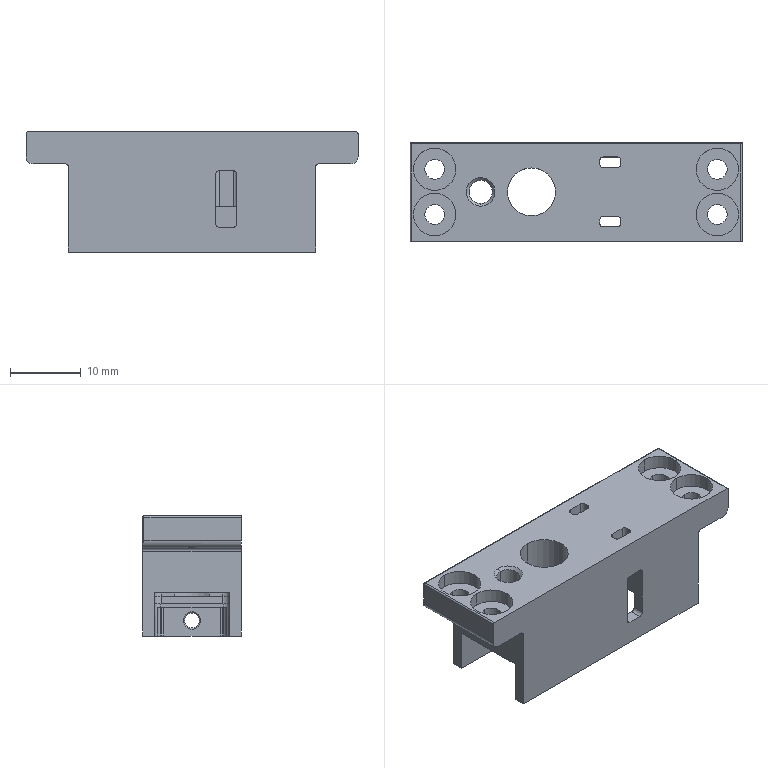NC program | NX | posted with a generic post | part box 47 x 14 x 17 mm
Lines 365 to 2938 of 2938, first 2161 of 2566 lines:
(ZLEVEL_PROFILE_COPY_1_COPY , TOOL : D1)
N686 T22 M6
N688 G54
N690 G17 G0 G90 X5.076 Y4.45 B0. C0. S9500 M3
N692 G43 Z30. H22
N694 Z1.
N696 G94 G1 X3.85 Z0.936 F1000.
N698 Y3.95 Z0.91
N700 X5.85 Z0.805
N702 Y4.45 Z0.779
N704 X3.85 Z0.674
N706 Y3.95 Z0.648
N708 X5.85 Z0.543
N710 Y4.45 Z0.516
N712 X3.85 Z0.412
N714 Y3.95 Z0.385
N716 X5.85 Z0.281
N718 Y4.45 Z0.254
N720 X3.85 Z0.15
N722 Y3.95 Z0.123
N724 X5.85 Z0.019
N726 Y4.45 Z-0.008
N728 X4.85 Z-0.06
N730 X3.85 F850.
N732 Y3.95
N734 X5.85
N736 Y4.45
N738 X4.85
N740 X3.85 Z-0.077
N742 Y4.075 Z-0.084
N744 X3.849 Y3.949 Z-0.086
N746 X3.931 Y3.95 Z-0.088
N748 X5.787 Z-0.12
N750 X5.85
N752 Y4.45
N754 X4.85
N756 X3.85 Z-0.137
N758 Y4.075 Z-0.144
N760 X3.849 Y3.949 Z-0.146
N762 X3.931 Y3.95 Z-0.148
N764 X5.787 Z-0.18
N766 X5.85
N768 Y4.45
N770 X4.85
N772 X3.85 Z-0.197
N774 Y4.075 Z-0.204
N776 X3.849 Y3.949 Z-0.206
N778 X3.931 Y3.95 Z-0.208
N780 X5.787 Z-0.24
N782 X5.85
N784 Y4.45
N786 X4.85
N788 X3.85 Z-0.257
N790 Y4.075 Z-0.264
N792 X3.849 Y3.949 Z-0.266
N794 X3.931 Y3.95 Z-0.268
N796 X5.787 Z-0.3
N798 X5.85
N800 Y4.45
N802 X4.85
N804 X3.85 Z-0.317
N806 Y4.075 Z-0.324
N808 X3.849 Y3.949 Z-0.326
N810 X3.931 Y3.95 Z-0.328
N812 X5.787 Z-0.36
N814 X5.85
N816 Y4.45
N818 X4.85
N820 X3.85 Z-0.377
N822 Y4.075 Z-0.384
N824 X3.849 Y3.949 Z-0.386
N826 X3.931 Y3.95 Z-0.388
N828 X5.787 Z-0.42
N830 X5.85
N832 Y4.45
N834 X4.85
N836 X3.85 Z-0.437
N838 Y4.075 Z-0.444
N840 X3.849 Y3.949 Z-0.446
N842 X3.931 Y3.95 Z-0.448
N844 X5.787 Z-0.48
N846 X5.85
N848 Y4.45
N850 X4.85
N852 X3.85 Z-0.497
N854 Y4.075 Z-0.504
N856 X3.849 Y3.949 Z-0.506
N858 X3.931 Y3.95 Z-0.508
N860 X5.787 Z-0.54
N862 X5.85
N864 Y4.45
N866 X4.85
N868 X3.85 Z-0.557
N870 Y4.075 Z-0.564
N872 X3.849 Y3.949 Z-0.566
N874 X3.931 Y3.95 Z-0.568
N876 X5.787 Z-0.6
N878 X5.85
N880 Y4.45
N882 X4.85
N884 X3.85 Z-0.617
N886 Y4.075 Z-0.624
N888 X3.849 Y3.949 Z-0.626
N890 X3.931 Y3.95 Z-0.628
N892 X5.787 Z-0.66
N894 X5.85
N896 Y4.45
N898 X4.85
N900 X3.85 Z-0.677
N902 Y4.075 Z-0.684
N904 X3.849 Y3.949 Z-0.686
N906 X3.931 Y3.95 Z-0.688
N908 X5.787 Z-0.72
N910 X5.85
N912 Y4.45
N914 X4.85
N916 X3.85 Z-0.737
N918 Y4.075 Z-0.744
N920 X3.849 Y3.949 Z-0.746
N922 X3.931 Y3.95 Z-0.748
N924 X5.787 Z-0.78
N926 X5.85
N928 Y4.45
N930 X4.85
N932 X3.85 Z-0.797
N934 Y4.075 Z-0.804
N936 X3.849 Y3.949 Z-0.806
N938 X3.931 Y3.95 Z-0.808
N940 X5.787 Z-0.84
N942 X5.85
N944 Y4.45
N946 X4.85
N948 X3.85 Z-0.857
N950 Y4.075 Z-0.864
N952 X3.849 Y3.949 Z-0.866
N954 X3.931 Y3.95 Z-0.868
N956 X5.787 Z-0.9
N958 X5.85
N960 Y4.45
N962 X4.85
N964 X3.85 Z-0.917
N966 Y4.075 Z-0.924
N968 X3.849 Y3.949 Z-0.926
N970 X3.931 Y3.95 Z-0.928
N972 X5.787 Z-0.96
N974 X5.85
N976 Y4.45
N978 X4.85
N980 X3.85 Z-0.977
N982 Y4.075 Z-0.984
N984 Y3.95 Z-0.986
N986 X3.931 Z-0.988
N988 X5.787 Z-1.02
N990 X5.85
N992 Y4.45
N994 X4.85
N996 X3.85 Z-1.037
N998 Y4.075 Z-1.044
N1000 Y3.95 Z-1.046
N1002 X3.931 Z-1.048
N1004 X5.787 Z-1.08
N1006 X5.85
N1008 Y4.45
N1010 X4.85
N1012 X3.85 Z-1.097
N1014 Y4.075 Z-1.104
N1016 Y3.95 Z-1.106
N1018 X3.931 Z-1.108
N1020 X5.787 Z-1.14
N1022 X5.85
N1024 Y4.45
N1026 X4.85
N1028 X3.85 Z-1.157
N1030 Y4.075 Z-1.164
N1032 Y3.95 Z-1.166
N1034 X3.931 Z-1.168
N1036 X5.787 Z-1.2
N1038 X5.85
N1040 Y4.45
N1042 X4.85
N1044 X3.85 Z-1.217
N1046 Y4.075 Z-1.224
N1048 Y3.95 Z-1.226
N1050 X3.931 Z-1.228
N1052 X5.787 Z-1.26
N1054 X5.84
N1056 X5.85 Y3.978
N1058 Y4.45
N1060 X4.85
N1062 X3.85 Z-1.277
N1064 Y4.075 Z-1.284
N1066 Y3.95 Z-1.286
N1068 X3.931 Z-1.288
N1070 X5.787 Z-1.32
N1072 X5.84
N1074 X5.85 Y3.978
N1076 Y4.45
N1078 X4.85
N1080 X3.85 Z-1.337
N1082 Y4.075 Z-1.344
N1084 Y3.95 Z-1.346
N1086 X3.931 Z-1.348
N1088 X5.787 Z-1.38
N1090 X5.84
N1092 X5.85 Y3.978
N1094 Y4.45
N1096 X4.85
N1098 X3.85 Z-1.397
N1100 Y4.075 Z-1.404
N1102 Y3.95 Z-1.406
N1104 X3.931 Z-1.408
N1106 X5.787 Z-1.44
N1108 X5.84
N1110 X5.85 Y3.978
N1112 Y4.45
N1114 X4.85
N1116 X3.85 Z-1.457
N1118 Y4.075 Z-1.464
N1120 Y3.95 Z-1.466
N1122 X3.931 Z-1.468
N1124 X5.787 Z-1.5
N1126 X5.84
N1128 X5.85 Y3.978
N1130 Y4.45
N1132 X4.85
N1134 X3.85 Z-1.517
N1136 Y4.075 Z-1.524
N1138 Y3.95 Z-1.526
N1140 X3.931 Z-1.528
N1142 X5.787 Z-1.56
N1144 X5.84
N1146 X5.85 Y3.978
N1148 Y4.45
N1150 X4.85
N1152 X3.85 Z-1.577
N1154 Y4.075 Z-1.584
N1156 Y3.95 Z-1.586
N1158 X3.931 Z-1.588
N1160 X5.787 Z-1.62
N1162 X5.84
N1164 X5.85 Y3.978
N1166 Y4.45
N1168 X4.85
N1170 X3.85 Z-1.637
N1172 Y4.075 Z-1.644
N1174 Y3.95 Z-1.646
N1176 X3.931 Z-1.648
N1178 X5.787 Z-1.68
N1180 X5.84
N1182 X5.85 Y3.978
N1184 Y4.45
N1186 X4.85
N1188 X3.85 Z-1.697
N1190 Y4.075 Z-1.704
N1192 Y3.95 Z-1.706
N1194 X3.931 Z-1.708
N1196 X5.787 Z-1.74
N1198 X5.84
N1200 X5.85 Y3.978
N1202 Y4.45
N1204 X4.85
N1206 X3.85 Z-1.757
N1208 Y4.075 Z-1.764
N1210 Y3.95 Z-1.766
N1212 X3.931 Z-1.768
N1214 X5.787 Z-1.8
N1216 X5.84
N1218 X5.85 Y3.978
N1220 Y4.45
N1222 X4.85
N1224 X3.85 Z-1.817
N1226 Y4.075 Z-1.824
N1228 Y3.95 Z-1.826
N1230 X3.931 Z-1.828
N1232 X5.787 Z-1.86
N1234 X5.84
N1236 X5.85 Y3.978
N1238 Y4.45
N1240 X4.85
N1242 X3.85 Z-1.877
N1244 Y4.075 Z-1.884
N1246 Y3.95 Z-1.886
N1248 X3.931 Z-1.888
N1250 X5.787 Z-1.92
N1252 X5.84
N1254 X5.85 Y3.978
N1256 Y4.45
N1258 X4.85
N1260 X3.85 Z-1.937
N1262 Y4.075 Z-1.944
N1264 Y3.95 Z-1.946
N1266 X3.931 Z-1.948
N1268 X5.787 Z-1.98
N1270 X5.84
N1272 X5.85 Y3.978
N1274 Y4.45
N1276 X4.85
N1278 X3.85 Z-1.997
N1280 Y4.075 Z-2.004
N1282 Y3.95 Z-2.006
N1284 X3.931 Z-2.008
N1286 X5.787 Z-2.04
N1288 X5.84
N1290 X5.85 Y3.978
N1292 Y4.45
N1294 X4.85
N1296 X3.85 Z-2.057
N1298 Y4.075 Z-2.064
N1300 Y3.95 Z-2.066
N1302 X3.931 Z-2.068
N1304 X5.787 Z-2.1
N1306 X5.84
N1308 X5.85 Y3.978
N1310 Y4.45
N1312 X4.85
N1314 X3.85 Z-2.117
N1316 Y4.075 Z-2.124
N1318 Y3.95 Z-2.126
N1320 X3.931 Z-2.128
N1322 X5.787 Z-2.16
N1324 X5.84
N1326 X5.85 Y3.978
N1328 Y4.45
N1330 X4.85
N1332 X3.85 Z-2.177
N1334 Y4.075 Z-2.184
N1336 Y3.95 Z-2.186
N1338 X3.931 Z-2.188
N1340 X5.787 Z-2.22
N1342 X5.84
N1344 X5.85 Y3.978
N1346 Y4.45
N1348 X4.85
N1350 X3.85 Z-2.237
N1352 Y4.075 Z-2.244
N1354 Y3.95 Z-2.246
N1356 X3.931 Z-2.248
N1358 X5.787 Z-2.28
N1360 X5.84
N1362 X5.85 Y3.978
N1364 Y4.45
N1366 X4.85
N1368 X3.85 Z-2.297
N1370 Y4.075 Z-2.304
N1372 Y3.95 Z-2.306
N1374 X3.931 Z-2.308
N1376 X5.787 Z-2.34
N1378 X5.84
N1380 X5.85 Y3.978
N1382 Y4.45
N1384 X4.85
N1386 X3.85 Z-2.357
N1388 Y4.075 Z-2.364
N1390 Y3.95 Z-2.366
N1392 X3.931 Z-2.368
N1394 X5.787 Z-2.4
N1396 X5.84
N1398 X5.85 Y3.978
N1400 Y4.45
N1402 X4.85
N1404 X3.85 Z-2.417
N1406 Y4.075 Z-2.424
N1408 Y3.95 Z-2.426
N1410 X3.931 Z-2.428
N1412 X5.787 Z-2.46
N1414 X5.84
N1416 X5.85 Y3.978
N1418 Y4.45
N1420 X4.85
N1422 X3.85 Z-2.477
N1424 Y4.075 Z-2.484
N1426 Y3.95 Z-2.486
N1428 X3.931 Z-2.488
N1430 X5.787 Z-2.52
N1432 X5.84
N1434 X5.85 Y3.978
N1436 Y4.45
N1438 X4.85
N1440 X3.85 Z-2.537
N1442 Y4.075 Z-2.544
N1444 Y3.95 Z-2.546
N1446 X3.931 Z-2.548
N1448 X5.787 Z-2.58
N1450 X5.84
N1452 X5.85 Y3.978
N1454 Y4.45
N1456 X4.85
N1458 X3.85 Z-2.597
N1460 Y4.075 Z-2.604
N1462 Y3.95 Z-2.606
N1464 X3.931 Z-2.608
N1466 X5.787 Z-2.64
N1468 X5.84
N1470 X5.85 Y3.978
N1472 Y4.45
N1474 X4.85
N1476 X3.85 Z-2.657
N1478 Y4.075 Z-2.664
N1480 Y3.95 Z-2.666
N1482 X3.931 Z-2.668
N1484 X5.787 Z-2.7
N1486 X5.84
N1488 X5.85 Y3.978
N1490 Y4.45
N1492 X4.85
N1494 X3.85 Z-2.717
N1496 Y4.075 Z-2.724
N1498 Y3.95 Z-2.726
N1500 X3.931 Z-2.728
N1502 X5.787 Z-2.76
N1504 X5.84
N1506 X5.85 Y3.978
N1508 Y4.45
N1510 X4.85
N1512 X3.85 Z-2.777
N1514 Y4.075 Z-2.784
N1516 Y3.95 Z-2.786
N1518 X3.931 Z-2.788
N1520 X5.787 Z-2.82
N1522 X5.84
N1524 X5.85 Y3.978
N1526 Y4.45
N1528 X4.85
N1530 X3.85 Z-2.837
N1532 Y4.075 Z-2.844
N1534 Y3.95 Z-2.846
N1536 X3.931 Z-2.848
N1538 X5.787 Z-2.88
N1540 X5.84
N1542 X5.85 Y3.978
N1544 Y4.45
N1546 X4.85
N1548 X3.85 Z-2.897
N1550 Y4.075 Z-2.904
N1552 Y3.95 Z-2.906
N1554 X3.931 Z-2.908
N1556 X5.787 Z-2.94
N1558 X5.84
N1560 X5.85 Y3.978
N1562 Y4.45
N1564 X4.85
N1566 X3.85 Z-2.957
N1568 Y4.075 Z-2.964
N1570 Y3.95 Z-2.966
N1572 X3.931 Z-2.968
N1574 X5.787 Z-3.
N1576 X5.84
N1578 X5.85 Y3.978
N1580 Y4.45
N1582 X4.85
N1584 X3.85 Z-3.017
N1586 Y4.075 Z-3.024
N1588 Y3.95 Z-3.026
N1590 X3.931 Z-3.028
N1592 X5.787 Z-3.06
N1594 X5.84
N1596 X5.85 Y3.978
N1598 Y4.45
N1600 X4.85
N1602 X3.85 Z-3.077
N1604 Y4.075 Z-3.084
N1606 Y3.95 Z-3.086
N1608 X3.931 Z-3.088
N1610 X5.787 Z-3.12
N1612 X5.84
N1614 X5.85 Y3.978
N1616 Y4.45
N1618 X4.85
N1620 X3.85 Z-3.137
N1622 Y4.075 Z-3.144
N1624 Y3.95 Z-3.146
N1626 X3.931 Z-3.148
N1628 X5.787 Z-3.18
N1630 X5.84
N1632 X5.85 Y3.978
N1634 Y4.45
N1636 X4.85
N1638 X3.85 Z-3.197
N1640 Y4.075 Z-3.204
N1642 Y3.95 Z-3.206
N1644 X3.931 Z-3.208
N1646 X5.787 Z-3.24
N1648 X5.84
N1650 X5.85 Y3.978
N1652 Y4.45
N1654 X4.85
N1656 X3.85 Z-3.257
N1658 Y4.075 Z-3.264
N1660 Y3.95 Z-3.266
N1662 X3.931 Z-3.268
N1664 X5.787 Z-3.3
N1666 X5.84
N1668 X5.85 Y3.978
N1670 Y4.45
N1672 X4.85
N1674 X3.85 Z-3.317
N1676 Y4.075 Z-3.324
N1678 Y3.95 Z-3.326
N1680 X3.931 Z-3.328
N1682 X5.787 Z-3.36
N1684 X5.84
N1686 X5.85 Y3.978
N1688 Y4.45
N1690 X4.85
N1692 X3.85 Z-3.377
N1694 Y4.075 Z-3.384
N1696 Y3.95 Z-3.386
N1698 X3.931 Z-3.388
N1700 X5.787 Z-3.42
N1702 X5.84
N1704 X5.85 Y3.978
N1706 Y4.45
N1708 X4.85
N1710 X3.85 Z-3.437
N1712 Y4.075 Z-3.444
N1714 Y3.95 Z-3.446
N1716 X3.931 Z-3.448
N1718 X5.787 Z-3.48
N1720 X5.84
N1722 X5.85 Y3.978
N1724 Y4.45
N1726 X4.85
N1728 X3.85 Z-3.497
N1730 Y4.075 Z-3.504
N1732 Y3.95 Z-3.506
N1734 X3.931 Z-3.508
N1736 X5.787 Z-3.54
N1738 X5.84
N1740 X5.85 Y3.978
N1742 Y4.45
N1744 X4.85
N1746 X3.85 Z-3.557
N1748 Y4.075 Z-3.564
N1750 Y3.95 Z-3.566
N1752 X3.931 Z-3.568
N1754 X5.787 Z-3.6
N1756 X5.84
N1758 X5.85 Y3.978
N1760 Y4.45
N1762 X4.85
N1764 X3.85 Z-3.617
N1766 Y4.075 Z-3.624
N1768 Y3.95 Z-3.626
N1770 X3.931 Z-3.628
N1772 X5.787 Z-3.66
N1774 X5.84
N1776 X5.85 Y3.978
N1778 Y4.45
N1780 X4.85
N1782 X3.85 Z-3.677
N1784 Y4.075 Z-3.684
N1786 Y3.95 Z-3.686
N1788 X3.931 Z-3.688
N1790 X5.787 Z-3.72
N1792 X5.84
N1794 X5.85 Y3.978
N1796 Y4.45
N1798 X4.85
N1800 X3.85 Z-3.737
N1802 Y4.075 Z-3.744
N1804 Y3.95 Z-3.746
N1806 X3.931 Z-3.748
N1808 X5.787 Z-3.78
N1810 X5.84
N1812 X5.85 Y3.978
N1814 Y4.45
N1816 X4.85
N1818 X3.85 Z-3.797
N1820 Y4.075 Z-3.804
N1822 Y3.95 Z-3.806
N1824 X3.931 Z-3.808
N1826 X5.787 Z-3.84
N1828 X5.84
N1830 X5.85 Y3.978
N1832 Y4.45
N1834 X4.85
N1836 X3.85 Z-3.857
N1838 Y4.075 Z-3.864
N1840 Y3.95 Z-3.866
N1842 X3.931 Z-3.868
N1844 X5.787 Z-3.9
N1846 X5.84
N1848 X5.85 Y3.978
N1850 Y4.45
N1852 X4.85
N1854 X3.85 Z-3.917
N1856 Y4.075 Z-3.924
N1858 Y3.95 Z-3.926
N1860 X3.931 Z-3.928
N1862 X5.787 Z-3.96
N1864 X5.84
N1866 X5.85 Y3.978
N1868 Y4.45
N1870 X4.85
N1872 X3.85 Z-3.977
N1874 Y4.075 Z-3.984
N1876 Y3.95 Z-3.986
N1878 X3.931 Z-3.988
N1880 X5.787 Z-4.02
N1882 X5.84
N1884 X5.85 Y3.978
N1886 Y4.45
N1888 X4.85
N1890 X3.85 Z-4.037
N1892 Y4.075 Z-4.044
N1894 Y3.95 Z-4.046
N1896 X3.931 Z-4.048
N1898 X5.787 Z-4.08
N1900 X5.84
N1902 X5.85 Y3.978
N1904 Y4.45
N1906 X4.85
N1908 X3.85 Z-4.097
N1910 Y4.075 Z-4.104
N1912 Y3.95 Z-4.106
N1914 X3.931 Z-4.108
N1916 X5.787 Z-4.14
N1918 X5.85
N1920 Y3.978
N1922 Y4.45
N1924 X4.85
N1926 X3.85 Z-4.157
N1928 Y4.075 Z-4.164
N1930 Y3.95 Z-4.166
N1932 X3.931 Z-4.168
N1934 X5.787 Z-4.2
N1936 X5.85
N1938 Y3.978
N1940 Y4.45
N1942 X4.85
N1944 X3.85 Z-4.217
N1946 Y4.075 Z-4.224
N1948 Y3.95 Z-4.226
N1950 X3.931 Z-4.228
N1952 X5.787 Z-4.26
N1954 X5.85
N1956 Y3.978
N1958 Y4.45
N1960 X4.85
N1962 X3.85 Z-4.277
N1964 Y4.075 Z-4.284
N1966 Y3.95 Z-4.286
N1968 X3.931 Z-4.288
N1970 X5.787 Z-4.32
N1972 X5.85
N1974 Y3.978
N1976 Y4.45
N1978 X4.85
N1980 X3.85 Z-4.337
N1982 Y4.075 Z-4.344
N1984 Y3.95 Z-4.346
N1986 X3.931 Z-4.348
N1988 X5.787 Z-4.38
N1990 X5.85
N1992 Y4.45
N1994 X4.85
N1996 X3.85 Z-4.397
N1998 Y4.075 Z-4.404
N2000 Y3.95 Z-4.406
N2002 X3.931 Z-4.408
N2004 X5.787 Z-4.44
N2006 X5.85
N2008 Y4.45
N2010 X4.85
N2012 X3.85 Z-4.457
N2014 Y4.075 Z-4.464
N2016 Y3.95 Z-4.466
N2018 X3.931 Z-4.468
N2020 X5.787 Z-4.5
N2022 X5.85
N2024 Y4.45
N2026 X4.85
N2028 X3.85 Z-4.517
N2030 Y4.075 Z-4.524
N2032 Y3.95 Z-4.526
N2034 X3.931 Z-4.528
N2036 X5.787 Z-4.56
N2038 X5.85
N2040 Y4.45
N2042 X4.85
N2044 X3.85 Z-4.577
N2046 Y4.075 Z-4.584
N2048 Y3.95 Z-4.586
N2050 X3.931 Z-4.588
N2052 X5.787 Z-4.62
N2054 X5.85
N2056 Y4.45
N2058 X4.85
N2060 X3.85 Z-4.637
N2062 Y4.075 Z-4.644
N2064 Y3.95 Z-4.646
N2066 X3.931 Z-4.648
N2068 X5.787 Z-4.68
N2070 X5.85
N2072 Y4.45
N2074 X4.85
N2076 X3.85 Z-4.697
N2078 Y4.075 Z-4.704
N2080 Y3.95 Z-4.706
N2082 X3.931 Z-4.708
N2084 X5.787 Z-4.74
N2086 X5.85
N2088 Y4.45
N2090 X4.85
N2092 X3.85 Z-4.757
N2094 Y4.075 Z-4.764
N2096 Y3.95 Z-4.766
N2098 X3.931 Z-4.768
N2100 X5.787 Z-4.8
N2102 X5.85
N2104 Y4.45
N2106 X4.85
N2108 X3.85 Z-4.817
N2110 Y4.075 Z-4.824
N2112 X3.851 Y3.951 Z-4.826
N2114 X3.931 Y3.95 Z-4.828
N2116 X5.787 Z-4.86
N2118 X5.85
N2120 Y4.45
N2122 X4.85
N2124 X3.85 Z-4.877
N2126 Y4.075 Z-4.884
N2128 X3.851 Y3.951 Z-4.886
N2130 X3.931 Y3.95 Z-4.888
N2132 X5.787 Z-4.92
N2134 X5.85
N2136 Y4.45
N2138 X4.85
N2140 X3.85 Z-4.937
N2142 Y4.075 Z-4.944
N2144 X3.851 Y3.951 Z-4.946
N2146 X3.931 Y3.95 Z-4.948
N2148 X5.787 Z-4.98
N2150 X5.85
N2152 Y4.45
N2154 X4.85
N2156 X3.85 Z-4.997
N2158 Y4.075 Z-5.004
N2160 X3.851 Y3.951 Z-5.006
N2162 X3.931 Y3.95 Z-5.008
N2164 X5.787 Z-5.04
N2166 X5.85
N2168 Y4.45
N2170 X4.85
N2172 X3.85 Z-5.057
N2174 Y4.075 Z-5.064
N2176 X3.851 Y3.951 Z-5.066
N2178 X3.931 Y3.95 Z-5.068
N2180 X5.787 Z-5.1
N2182 X5.85
N2184 Y4.45
N2186 X4.85
N2188 X3.85 Z-5.117
N2190 Y4.075 Z-5.124
N2192 X3.851 Y3.951 Z-5.126
N2194 X3.931 Y3.95 Z-5.128
N2196 X5.787 Z-5.16
N2198 X5.85
N2200 Y4.45
N2202 X4.85
N2204 X3.85 Z-5.177
N2206 Y4.075 Z-5.184
N2208 X3.851 Y3.951 Z-5.186
N2210 X3.931 Y3.95 Z-5.188
N2212 X5.787 Z-5.22
N2214 X5.85
N2216 Y4.45
N2218 X4.85
N2220 X3.85 Z-5.237
N2222 Y4.075 Z-5.244
N2224 X3.851 Y3.951 Z-5.246
N2226 X3.931 Y3.95 Z-5.248
N2228 X5.787 Z-5.28
N2230 X5.85
N2232 Y4.45
N2234 X4.85
N2236 X3.85 Z-5.297
N2238 Y4.075 Z-5.304
N2240 X3.851 Y3.951 Z-5.306
N2242 X3.931 Y3.95 Z-5.308
N2244 X5.787 Z-5.34
N2246 X5.85
N2248 Y4.45
N2250 X4.85
N2252 X3.85 Z-5.357
N2254 Y4.075 Z-5.364
N2256 X3.851 Y3.951 Z-5.366
N2258 X3.931 Y3.95 Z-5.368
N2260 X5.787 Z-5.4
N2262 X5.85
N2264 Y4.45
N2266 X4.85
N2268 X3.85 Z-5.417
N2270 Y4.075 Z-5.424
N2272 X3.851 Y3.951 Z-5.426
N2274 X3.931 Y3.95 Z-5.428
N2276 X5.787 Z-5.46
N2278 X5.85
N2280 Y4.45
N2282 X4.85
N2284 X3.85 Z-5.477
N2286 Y4.075 Z-5.484
N2288 X3.851 Y3.951 Z-5.486
N2290 X3.931 Y3.95 Z-5.488
N2292 X5.787 Z-5.52
N2294 X5.85
N2296 Y4.45
N2298 X4.85
N2300 X3.85 Z-5.537
N2302 Y4.075 Z-5.544
N2304 X3.851 Y3.951 Z-5.546
N2306 X3.931 Y3.95 Z-5.548
N2308 X5.788 Z-5.58
N2310 X5.85
N2312 Y4.45
N2314 X4.85
N2316 X3.85 Z-5.597
N2318 Y4.075 Z-5.604
N2320 X3.851 Y3.951 Z-5.606
N2322 X3.931 Y3.95 Z-5.608
N2324 X5.788 Z-5.64
N2326 X5.85
N2328 Y4.45
N2330 X4.85
N2332 X3.85 Z-5.657
N2334 Y4.075 Z-5.664
N2336 X3.851 Y3.951 Z-5.666
N2338 X3.931 Y3.95 Z-5.668
N2340 X5.788 Z-5.7
N2342 X5.85
N2344 Y4.45
N2346 X4.85
N2348 X3.85 Z-5.717
N2350 Y4.075 Z-5.724
N2352 X3.851 Y3.951 Z-5.726
N2354 X3.931 Y3.95 Z-5.728
N2356 X5.788 Z-5.76
N2358 X5.85
N2360 Y4.45
N2362 X4.85
N2364 X3.85 Z-5.777
N2366 Y4.075 Z-5.784
N2368 X3.851 Y3.951 Z-5.786
N2370 X3.931 Y3.95 Z-5.788
N2372 X5.788 Z-5.82
N2374 X5.85
N2376 Y4.45
N2378 X4.85
N2380 X3.85 Z-5.837
N2382 Y4.075 Z-5.844
N2384 X3.851 Y3.951 Z-5.846
N2386 X3.931 Y3.95 Z-5.848
N2388 X5.788 Z-5.88
N2390 X5.85
N2392 Y4.45
N2394 X4.85
N2396 X3.85 Z-5.897
N2398 Y4.075 Z-5.904
N2400 X3.851 Y3.951 Z-5.906
N2402 X3.931 Y3.95 Z-5.908
N2404 X5.788 Z-5.94
N2406 X5.85
N2408 Y4.45
N2410 X4.85
N2412 X3.85 Z-5.957
N2414 Y4.075 Z-5.964
N2416 X3.851 Y3.951 Z-5.966
N2418 X3.931 Y3.95 Z-5.968
N2420 X5.788 Z-6.
N2422 X5.85
N2424 Y4.45
N2426 X4.85
N2428 X3.85 Z-6.017
N2430 Y4.075 Z-6.024
N2432 X3.851 Y3.951 Z-6.026
N2434 X3.931 Y3.95 Z-6.028
N2436 X5.788 Z-6.06
N2438 X5.85
N2440 Y4.45
N2442 X4.85
N2444 X3.85 Z-6.077
N2446 Y4.075 Z-6.084
N2448 X3.851 Y3.951 Z-6.086
N2450 X3.931 Y3.95 Z-6.088
N2452 X5.788 Z-6.12
N2454 X5.85
N2456 Y4.45
N2458 X4.85
N2460 X3.85 Z-6.137
N2462 Y4.075 Z-6.144
N2464 X3.851 Y3.951 Z-6.146
N2466 X3.931 Y3.95 Z-6.148
N2468 X5.788 Z-6.18
N2470 X5.85
N2472 Y4.45
N2474 X4.85
N2476 X3.85 Z-6.197
N2478 Y4.075 Z-6.204
N2480 X3.851 Y3.951 Z-6.206
N2482 X3.931 Y3.95 Z-6.208
N2484 X5.788 Z-6.24
N2486 X5.85
N2488 Y4.45
N2490 X4.85
N2492 X3.85 Z-6.257
N2494 Y4.075 Z-6.264
N2496 X3.851 Y3.951 Z-6.266
N2498 X3.931 Y3.95 Z-6.268
N2500 X5.788 Z-6.3
N2502 X5.85
N2504 Y4.45
N2506 X4.85
N2508 X3.85 Z-6.317
N2510 Y4.075 Z-6.324
N2512 X3.851 Y3.951 Z-6.326
N2514 X3.931 Y3.95 Z-6.328
N2516 X5.788 Z-6.36
N2518 X5.85
N2520 Y4.45
N2522 X4.85
N2524 X3.85 Z-6.377
N2526 Y4.075 Z-6.384
N2528 X3.851 Y3.951 Z-6.386
N2530 X3.931 Y3.95 Z-6.388
N2532 X5.788 Z-6.42
N2534 X5.85
N2536 Y4.45
N2538 X4.85
N2540 X3.85 Z-6.437
N2542 Y4.075 Z-6.444
N2544 X3.851 Y3.951 Z-6.446
N2546 X3.931 Y3.95 Z-6.448
N2548 X5.788 Z-6.48
N2550 X5.85
N2552 Y4.45
N2554 X4.85
N2556 X3.85 Z-6.497
N2558 Y4.075 Z-6.504
N2560 X3.851 Y3.951 Z-6.506
N2562 X3.931 Y3.95 Z-6.508
N2564 X5.788 Z-6.54
N2566 X5.85
N2568 Y4.45
N2570 X4.85
N2572 X3.85 Z-6.557
N2574 Y4.075 Z-6.564
N2576 X3.851 Y3.951 Z-6.566
N2578 X3.931 Y3.95 Z-6.568
N2580 X5.788 Z-6.6
N2582 X5.85
N2584 Y4.45
N2586 X4.85
N2588 X3.85 Z-6.617
N2590 Y4.075 Z-6.624
N2592 X3.851 Y3.951 Z-6.626
N2594 X3.931 Y3.95 Z-6.628
N2596 X5.788 Z-6.66
N2598 X5.85
N2600 Y4.45
N2602 X4.85
N2604 X3.85 Z-6.677
N2606 Y4.075 Z-6.684
N2608 X3.851 Y3.951 Z-6.686
N2610 X3.931 Y3.95 Z-6.688
N2612 X5.788 Z-6.72
N2614 X5.85
N2616 Y4.45
N2618 X4.85
N2620 X3.85 Z-6.737
N2622 Y4.075 Z-6.744
N2624 X3.851 Y3.951 Z-6.746
N2626 X3.931 Y3.95 Z-6.748
N2628 X5.788 Z-6.78
N2630 X5.85
N2632 Y4.45
N2634 X4.85
N2636 X3.85 Z-6.797
N2638 Y4.075 Z-6.804
N2640 X3.851 Y3.951 Z-6.806
N2642 X3.931 Y3.95 Z-6.808
N2644 X5.788 Z-6.84
N2646 X5.85
N2648 Y4.45
N2650 X4.85
N2652 X3.85 Z-6.857
N2654 Y4.075 Z-6.864
N2656 X3.851 Y3.951 Z-6.866
N2658 X3.931 Y3.95 Z-6.868
N2660 X5.788 Z-6.9
N2662 X5.85
N2664 Y4.45
N2666 X4.85
N2668 X3.85 Z-6.917
N2670 Y4.075 Z-6.924
N2672 X3.851 Y3.951 Z-6.926
N2674 X3.931 Y3.95 Z-6.928
N2676 X5.788 Z-6.96
N2678 X5.849
N2680 X5.85 Y4.45
N2682 X4.85
N2684 X3.85 Z-6.977
N2686 Y4.075 Z-6.984
N2688 X3.851 Y3.951 Z-6.986
N2690 X3.931 Y3.95 Z-6.988
N2692 X5.788 Z-7.02
N2694 X5.849
N2696 X5.85 Y4.45
N2698 X4.85
N2700 X3.85 Z-7.037
N2702 Y4.075 Z-7.044
N2704 X3.851 Y3.951 Z-7.046
N2706 X3.931 Y3.95 Z-7.048
N2708 X5.788 Z-7.08
N2710 X5.849
N2712 X5.85 Y4.45
N2714 X4.85
N2716 X3.85 Z-7.097
N2718 Y4.075 Z-7.104
N2720 X3.851 Y3.951 Z-7.106
N2722 X3.931 Y3.95 Z-7.108
N2724 X5.788 Z-7.14
N2726 X5.849
N2728 X5.85 Y4.45
N2730 X4.85
N2732 X3.85 Z-7.157
N2734 Y4.075 Z-7.164
N2736 X3.851 Y3.951 Z-7.166
N2738 X3.931 Y3.95 Z-7.168
N2740 X5.788 Z-7.2
N2742 X5.849
N2744 X5.85 Y4.45
N2746 X4.85
N2748 X3.85 Z-7.217
N2750 Y4.075 Z-7.224
N2752 X3.851 Y3.951 Z-7.226
N2754 X3.931 Y3.95 Z-7.228
N2756 X5.788 Z-7.26
N2758 X5.849
N2760 X5.85 Y4.45
N2762 X4.85
N2764 X3.85 Z-7.277
N2766 Y4.075 Z-7.284
N2768 X3.851 Y3.951 Z-7.286
N2770 X3.931 Y3.95 Z-7.288
N2772 X5.788 Z-7.32
N2774 X5.849
N2776 X5.85 Y4.45
N2778 X4.85
N2780 X3.85 Z-7.337
N2782 Y4.075 Z-7.344
N2784 X3.851 Y3.951 Z-7.346
N2786 X3.931 Y3.95 Z-7.348
N2788 X5.788 Z-7.38
N2790 X5.85
N2792 Y4.45
N2794 X4.85
N2796 X3.85 Z-7.397
N2798 Y4.075 Z-7.404
N2800 X3.851 Y3.951 Z-7.406
N2802 X3.932 Y3.95 Z-7.408
N2804 X5.788 Z-7.44
N2806 X5.85
N2808 Y4.45
N2810 X4.85
N2812 X3.85 Z-7.457
N2814 Y4.075 Z-7.464
N2816 X3.851 Y3.951 Z-7.466
N2818 X3.932 Y3.95 Z-7.468
N2820 X5.788 Z-7.5
N2822 X5.85
N2824 Y4.45
N2826 X4.85
N2828 X3.85 Z-7.517
N2830 Y4.075 Z-7.524
N2832 X3.851 Y3.951 Z-7.526
N2834 X3.932 Y3.95 Z-7.528
N2836 X5.788 Z-7.56
N2838 X5.85
N2840 Y4.45
N2842 X4.85
N2844 X3.85 Z-7.577
N2846 Y4.075 Z-7.584
N2848 X3.851 Y3.951 Z-7.586
N2850 X3.932 Y3.95 Z-7.588
N2852 X5.788 Z-7.62
N2854 X5.85
N2856 Y4.45
N2858 X4.85
N2860 X3.85 Z-7.637
N2862 Y4.075 Z-7.644
N2864 X3.851 Y3.951 Z-7.646
N2866 X3.932 Y3.95 Z-7.648
N2868 X5.788 Z-7.68
N2870 X5.85 Y3.951
N2872 Y4.45
N2874 X4.85
N2876 X3.85 Z-7.697
N2878 Y4.075 Z-7.704
N2880 X3.851 Y3.951 Z-7.706
N2882 X3.932 Y3.95 Z-7.708
N2884 X5.788 Z-7.74
N2886 X5.85 Y3.951
N2888 Y4.45
N2890 X4.85
N2892 X3.85 Z-7.757
N2894 Y4.075 Z-7.764
N2896 X3.851 Y3.951 Z-7.766
N2898 X3.932 Y3.95 Z-7.768
N2900 X5.788 Z-7.8
N2902 X5.85 Y3.951
N2904 Y4.45
N2906 X4.85
N2908 X3.85 Z-7.817
N2910 Y4.075 Z-7.824
N2912 X3.851 Y3.951 Z-7.826
N2914 X3.932 Y3.95 Z-7.828
N2916 X5.788 Z-7.86
N2918 X5.85 Y3.951
N2920 Y4.45
N2922 X4.85
N2924 X3.85 Z-7.877
N2926 Y4.075 Z-7.884
N2928 X3.851 Y3.951 Z-7.886
N2930 X3.932 Y3.95 Z-7.888
N2932 X5.788 Z-7.92
N2934 X5.85 Y3.951
N2936 Y4.45
N2938 X4.85
N2940 X3.85 Z-7.937
N2942 Y4.075 Z-7.944
N2944 X3.851 Y3.951 Z-7.946
N2946 X3.932 Y3.95 Z-7.948
N2948 X5.788 Z-7.98
N2950 X5.85 Y3.951
N2952 Y4.45
N2954 X4.85
N2956 X3.85 Z-7.997
N2958 Y4.075 Z-8.004
N2960 X3.851 Y3.951 Z-8.006
N2962 X3.932 Y3.95 Z-8.008
N2964 X5.788 Z-8.04
N2966 X5.85 Y3.951
N2968 Y4.45
N2970 X4.85
N2972 X3.85 Z-8.057
N2974 Y4.075 Z-8.064
N2976 X3.851 Y3.951 Z-8.066
N2978 X3.932 Y3.95 Z-8.068
N2980 X5.788 Z-8.1
N2982 X5.85 Y3.951
N2984 Y4.45
N2986 X4.85
N2988 X3.85 Z-8.117
N2990 Y4.075 Z-8.124
N2992 X3.851 Y3.951 Z-8.126
N2994 X3.932 Y3.95 Z-8.128
N2996 X5.788 Z-8.16
N2998 X5.85 Y3.951
N3000 Y4.45
N3002 X4.85
N3004 X3.85 Z-8.177
N3006 Y4.075 Z-8.184
N3008 X3.851 Y3.951 Z-8.186
N3010 X3.932 Y3.95 Z-8.188
N3012 X5.788 Z-8.22
N3014 X5.85 Y3.951
N3016 Y4.45
N3018 X4.85
N3020 X3.85 Z-8.237
N3022 Y4.075 Z-8.244
N3024 X3.851 Y3.951 Z-8.246
N3026 X3.932 Y3.95 Z-8.248
N3028 X5.788 Z-8.28
N3030 X5.85 Y3.951
N3032 Y4.45
N3034 X4.85
N3036 X3.85 Z-8.297
N3038 Y4.075 Z-8.304
N3040 X3.851 Y3.951 Z-8.306
N3042 X3.932 Y3.95 Z-8.308
N3044 X5.788 Z-8.34
N3046 X5.85 Y3.951
N3048 Y4.45
N3050 X4.85
N3052 X3.85 Z-8.357
N3054 Y4.075 Z-8.364
N3056 X3.851 Y3.951 Z-8.366
N3058 X3.932 Y3.95 Z-8.368
N3060 X5.788 Z-8.4
N3062 X5.85 Y3.951
N3064 Y4.45
N3066 X4.85
N3068 X3.85 Z-8.417
N3070 Y4.075 Z-8.424
N3072 X3.851 Y3.951 Z-8.426
N3074 X3.932 Y3.95 Z-8.428
N3076 X5.788 Z-8.46
N3078 X5.85 Y3.951
N3080 Y4.45
N3082 X4.85
N3084 X3.85 Z-8.477
N3086 Y4.075 Z-8.484
N3088 X3.851 Y3.951 Z-8.486
N3090 X3.932 Y3.95 Z-8.488
N3092 X5.788 Z-8.52
N3094 X5.85 Y3.951
N3096 Y4.45
N3098 X4.85
N3100 X3.85 Z-8.537
N3102 Y4.075 Z-8.544
N3104 X3.851 Y3.951 Z-8.546
N3106 X3.932 Y3.95 Z-8.548
N3108 X5.788 Z-8.58
N3110 X5.85 Y3.951
N3112 Y4.45
N3114 X4.85
N3116 X3.85 Z-8.597
N3118 Y4.075 Z-8.604
N3120 X3.851 Y3.951 Z-8.606
N3122 X3.932 Y3.95 Z-8.608
N3124 X5.788 Z-8.64
N3126 X5.85 Y3.951
N3128 Y4.45
N3130 X4.85
N3132 X3.85 Z-8.657
N3134 Y4.075 Z-8.664
N3136 X3.851 Y3.951 Z-8.666
N3138 X3.932 Y3.95 Z-8.668
N3140 X5.788 Z-8.7
N3142 X5.85 Y3.951
N3144 Y4.45
N3146 X4.85
N3148 X3.85 Z-8.717
N3150 Y4.075 Z-8.724
N3152 X3.851 Y3.951 Z-8.726
N3154 X3.932 Y3.95 Z-8.728
N3156 X5.788 Z-8.76
N3158 X5.85 Y3.951
N3160 Y4.45
N3162 X4.85
N3164 X3.85 Z-8.777
N3166 Y4.075 Z-8.784
N3168 X3.851 Y3.951 Z-8.786
N3170 X3.932 Y3.95 Z-8.788
N3172 X5.788 Z-8.82
N3174 X5.85 Y3.951
N3176 Y4.45
N3178 X4.85
N3180 X3.85 Z-8.837
N3182 Y4.075 Z-8.844
N3184 X3.851 Y3.951 Z-8.846
N3186 X3.932 Y3.95 Z-8.848
N3188 X5.788 Z-8.88
N3190 X5.85 Y3.951
N3192 Y4.45
N3194 X4.85
N3196 X3.85 Z-8.897
N3198 Y4.075 Z-8.904
N3200 X3.851 Y3.951 Z-8.906
N3202 X3.932 Y3.95 Z-8.908
N3204 X5.788 Z-8.94
N3206 X5.85 Y3.951
N3208 Y4.45
N3210 X4.85
N3212 X3.85 Z-8.957
N3214 Y4.075 Z-8.964
N3216 X3.851 Y3.951 Z-8.966
N3218 X3.932 Y3.95 Z-8.968
N3220 X5.788 Z-9.
N3222 X5.85 Y3.951
N3224 Y4.45
N3226 X4.85
N3228 X3.85 Z-9.017
N3230 Y4.075 Z-9.024
N3232 X3.851 Y3.951 Z-9.026
N3234 X3.932 Y3.95 Z-9.028
N3236 X5.788 Z-9.06
N3238 X5.85 Y3.951
N3240 Y4.45
N3242 X4.85
N3244 X3.85 Z-9.077
N3246 Y4.075 Z-9.084
N3248 X3.851 Y3.951 Z-9.086
N3250 X3.932 Y3.95 Z-9.088
N3252 X5.788 Z-9.12
N3254 X5.85 Y3.951
N3256 Y4.45
N3258 X4.85
N3260 X3.85 Z-9.137
N3262 Y4.075 Z-9.144
N3264 X3.851 Y3.951 Z-9.146
N3266 X3.932 Y3.95 Z-9.148
N3268 X5.788 Z-9.18
N3270 X5.85 Y3.951
N3272 Y4.45
N3274 X4.85
N3276 X3.85 Z-9.197
N3278 Y4.075 Z-9.204
N3280 X3.851 Y3.951 Z-9.206
N3282 X3.932 Y3.95 Z-9.208
N3284 X5.788 Z-9.24
N3286 X5.85 Y3.951
N3288 Y4.45
N3290 X4.85
N3292 X3.85 Z-9.257
N3294 Y4.075 Z-9.264
N3296 X3.851 Y3.951 Z-9.266
N3298 X3.932 Y3.95 Z-9.268
N3300 X5.788 Z-9.3
N3302 X5.85 Y3.951
N3304 Y4.45
N3306 X4.85
N3308 X3.85 Z-9.317
N3310 Y4.075 Z-9.324
N3312 X3.851 Y3.951 Z-9.326
N3314 X3.932 Y3.95 Z-9.328
N3316 X5.788 Z-9.36
N3318 X5.85 Y3.951
N3320 Y4.45
N3322 X4.85
N3324 X3.85 Z-9.377
N3326 Y4.075 Z-9.384
N3328 X3.851 Y3.951 Z-9.386
N3330 X3.932 Y3.95 Z-9.388
N3332 X5.788 Z-9.42
N3334 X5.85 Y3.951
N3336 Y4.45
N3338 X4.85
N3340 X3.85 Z-9.437
N3342 Y4.075 Z-9.444
N3344 X3.851 Y3.951 Z-9.446
N3346 X3.932 Y3.95 Z-9.448
N3348 X5.788 Z-9.48
N3350 X5.85 Y3.951
N3352 Y4.45
N3354 X4.85
N3356 X3.85 Z-9.497
N3358 Y4.075 Z-9.504
N3360 X3.851 Y3.951 Z-9.506
N3362 X3.932 Y3.95 Z-9.508
N3364 X5.788 Z-9.54
N3366 X5.849
N3368 X5.85 Y4.45
N3370 X4.85
N3372 X3.85 Z-9.557
N3374 Y4.075 Z-9.564
N3376 X3.851 Y3.951 Z-9.566
N3378 X3.932 Y3.95 Z-9.568
N3380 X5.788 Z-9.6
N3382 X5.849
N3384 X5.85 Y4.45
N3386 X4.85
N3388 X3.85 Z-9.617
N3390 Y4.075 Z-9.624
N3392 X3.851 Y3.951 Z-9.626
N3394 X3.932 Y3.95 Z-9.628
N3396 X5.788 Z-9.66
N3398 X5.849
N3400 X5.85 Y4.45
N3402 X4.85
N3404 X3.85 Z-9.677
N3406 Y4.075 Z-9.684
N3408 X3.851 Y3.951 Z-9.686
N3410 X3.932 Y3.95 Z-9.688
N3412 X5.788 Z-9.72
N3414 X5.849
N3416 X5.85 Y4.45
N3418 X4.85
N3420 X3.85 Z-9.737
N3422 Y4.075 Z-9.744
N3424 X3.851 Y3.951 Z-9.746
N3426 X3.932 Y3.95 Z-9.748
N3428 X5.788 Z-9.78
N3430 X5.849
N3432 X5.85 Y4.45
N3434 X4.85
N3436 X3.85 Z-9.797
N3438 Y4.075 Z-9.804
N3440 X3.851 Y3.951 Z-9.806
N3442 X3.932 Y3.95 Z-9.808
N3444 X5.788 Z-9.84
N3446 X5.849
N3448 X5.85 Y4.45
N3450 X4.85
N3452 X3.85 Z-9.857
N3454 Y4.075 Z-9.864
N3456 X3.851 Y3.951 Z-9.866
N3458 X3.932 Y3.95 Z-9.868
N3460 X5.788 Z-9.9
N3462 X5.849
N3464 X5.85 Y4.45
N3466 X4.85
N3468 X3.85 Z-9.917
N3470 Y4.075 Z-9.924
N3472 X3.851 Y3.951 Z-9.926
N3474 X3.932 Y3.95 Z-9.928
N3476 X5.788 Z-9.96
N3478 X5.849
N3480 X5.85 Y3.971
N3482 Y4.45
N3484 X4.85
N3486 X3.85 Z-9.977
N3488 Y4.075 Z-9.984
N3490 X3.851 Y3.951 Z-9.986
N3492 X3.932 Y3.95 Z-9.988
N3494 X5.788 Z-10.02
N3496 X5.849
N3498 X5.85 Y3.974
N3500 Y4.45
N3502 X4.85
N3504 X3.85 Z-10.037
N3506 Y4.075 Z-10.044
N3508 X3.851 Y3.951 Z-10.046
N3510 X3.932 Y3.95 Z-10.048
N3512 X5.788 Z-10.08
N3514 X5.849
N3516 X5.85 Y3.977
N3518 Y4.45
N3520 X4.85
N3522 X3.85 Z-10.097
N3524 Y4.075 Z-10.104
N3526 X3.851 Y3.951 Z-10.106
N3528 X3.932 Y3.95 Z-10.108
N3530 X5.788 Z-10.14
N3532 X5.849
N3534 X5.85 Y3.978
N3536 Y4.45
N3538 X4.85
N3540 X3.85 Z-10.157
N3542 Y4.075 Z-10.164
N3544 X3.851 Y3.951 Z-10.166
N3546 X3.932 Y3.95 Z-10.168
N3548 X5.788 Z-10.2
N3550 X5.849
N3552 X5.85 Y3.978
N3554 Y4.45
N3556 X4.85
N3558 X3.85 Z-10.217
N3560 Y4.075 Z-10.224
N3562 X3.851 Y3.951 Z-10.226
N3564 X3.932 Y3.95 Z-10.228
N3566 X5.788 Z-10.26
N3568 X5.85 Y3.951
N3570 Y4.45
N3572 X4.85
N3574 X3.85 Z-10.277
N3576 Y4.075 Z-10.284
N3578 X3.851 Y3.951 Z-10.286
N3580 X3.932 Y3.95 Z-10.288
N3582 X5.788 Z-10.32
N3584 X5.85 Y3.951
N3586 Y4.45
N3588 X4.85
N3590 X3.85 Z-10.337
N3592 Y4.075 Z-10.344
N3594 X3.851 Y3.951 Z-10.346
N3596 X3.932 Y3.95 Z-10.348
N3598 X5.788 Z-10.38
N3600 X5.85 Y3.951
N3602 Y4.45
N3604 X4.85
N3606 X3.85 Z-10.397
N3608 Y4.075 Z-10.404
N3610 X3.851 Y3.951 Z-10.406
N3612 X3.932 Y3.95 Z-10.408
N3614 X5.788 Z-10.44
N3616 X5.85 Y3.951
N3618 Y4.45
N3620 X4.85
N3622 X3.85 Z-10.457
N3624 Y4.075 Z-10.464
N3626 X3.851 Y3.951 Z-10.466
N3628 X3.932 Y3.95 Z-10.468
N3630 X5.788 Z-10.5
N3632 X5.85 Y3.951
N3634 Y4.45
N3636 X3.85
N3638 X3.851 Y3.95
N3640 X5.788
N3642 X5.818 Y3.948
N3644 X5.831 Y3.975
N3646 Z-10.4
N3648 G0 Z30.
(ZLEVEL_PROFILE_COPY_1_COPY_COPY , TOOL : D1)
N3650 X4.624 Y-4.45
N3652 Z1.
N3654 G1 X5.85 Z0.936 F1000.
N3656 Y-3.95 Z0.91
N3658 X3.85 Z0.805
N3660 Y-4.45 Z0.779
N3662 X3.899 Z0.776
N3664 X5.85 Z0.674
N3666 Y-3.95 Z0.648
N3668 X3.85 Z0.543
N3670 Y-4.45 Z0.516
N3672 X3.899 Z0.514
N3674 X5.85 Z0.412
N3676 Y-3.95 Z0.385
N3678 X3.85 Z0.281
N3680 Y-4.45 Z0.254
N3682 X3.899 Z0.252
N3684 X5.85 Z0.15
N3686 Y-3.95 Z0.123
N3688 X3.85 Z0.019
N3690 Y-4.45 Z-0.008
N3692 X3.899 Z-0.01
N3694 X4.85 Z-0.06
N3696 X5.85 F850.
N3698 Y-3.95
N3700 X3.85
N3702 Y-4.45
N3704 X3.899
N3706 X4.85
N3708 X5.85 Z-0.077
N3710 Y-4.075 Z-0.084
N3712 X5.849 Y-3.95 Z-0.086
N3714 X5.769 Z-0.088
N3716 X3.913 Z-0.12
N3718 X3.85
N3720 Y-4.45
N3722 X3.899
N3724 X4.85
N3726 X5.85 Z-0.137
N3728 Y-4.075 Z-0.144
N3730 X5.849 Y-3.95 Z-0.146
N3732 X5.769 Z-0.148
N3734 X3.913 Z-0.18
N3736 X3.85
N3738 Y-4.45
N3740 X3.899
N3742 X4.85
N3744 X5.85 Z-0.197
N3746 Y-4.075 Z-0.204
N3748 X5.849 Y-3.95 Z-0.206
N3750 X5.769 Z-0.208
N3752 X3.913 Z-0.24
N3754 X3.85
N3756 Y-4.45
N3758 X3.899
N3760 X4.85
N3762 X5.85 Z-0.257
N3764 Y-4.075 Z-0.264
N3766 X5.849 Y-3.95 Z-0.266
N3768 X5.769 Z-0.268
N3770 X3.913 Z-0.3
N3772 X3.85
N3774 Y-4.45
N3776 X3.899
N3778 X4.85
N3780 X5.85 Z-0.317
N3782 Y-4.075 Z-0.324
N3784 X5.849 Y-3.95 Z-0.326
N3786 X5.769 Z-0.328
N3788 X3.913 Z-0.36
N3790 X3.85
N3792 Y-4.45
N3794 X3.899
N3796 X4.85
N3798 X5.85 Z-0.377
N3800 Y-4.075 Z-0.384
N3802 X5.849 Y-3.95 Z-0.386
N3804 X5.769 Z-0.388
N3806 X3.913 Z-0.42
N3808 X3.85
N3810 Y-4.45
N3812 X3.899
N3814 X4.85
N3816 X5.85 Z-0.437
N3818 Y-4.075 Z-0.444
N3820 X5.849 Y-3.95 Z-0.446
N3822 X5.769 Z-0.448
N3824 X3.913 Z-0.48
N3826 X3.85
N3828 Y-4.45
N3830 X3.899
N3832 X4.85
N3834 X5.85 Z-0.497
N3836 Y-4.075 Z-0.504
N3838 X5.849 Y-3.95 Z-0.506
N3840 X5.769 Z-0.508
N3842 X3.913 Z-0.54
N3844 X3.85
N3846 Y-4.45
N3848 X3.899
N3850 X4.85
N3852 X5.85 Z-0.557
N3854 Y-4.075 Z-0.564
N3856 X5.849 Y-3.95 Z-0.566
N3858 X5.769 Z-0.568
N3860 X3.913 Z-0.6
N3862 X3.85
N3864 Y-4.45
N3866 X3.899
N3868 X4.85
N3870 X5.85 Z-0.617
N3872 Y-4.075 Z-0.624
N3874 X5.849 Y-3.95 Z-0.626
N3876 X5.769 Z-0.628
N3878 X3.913 Z-0.66
N3880 X3.85
N3882 Y-4.45
N3884 X3.899
N3886 X4.85
N3888 X5.85 Z-0.677
N3890 Y-4.075 Z-0.684
N3892 X5.849 Y-3.95 Z-0.686
N3894 X5.769 Z-0.688
N3896 X3.913 Z-0.72
N3898 X3.85
N3900 Y-4.45
N3902 X3.899
N3904 X4.85
N3906 X5.85 Z-0.737
N3908 Y-4.075 Z-0.744
N3910 X5.849 Y-3.95 Z-0.746
N3912 X5.769 Z-0.748
N3914 X3.913 Z-0.78
N3916 X3.85
N3918 Y-4.45
N3920 X3.899
N3922 X4.85
N3924 X5.85 Z-0.797
N3926 Y-4.075 Z-0.804
N3928 X5.849 Y-3.95 Z-0.806
N3930 X5.769 Z-0.808
N3932 X3.913 Z-0.84
N3934 X3.85
N3936 Y-4.45
N3938 X3.899
N3940 X4.85
N3942 X5.85 Z-0.857
N3944 Y-4.075 Z-0.864
N3946 X5.849 Y-3.95 Z-0.866
N3948 X5.769 Z-0.868
N3950 X3.913 Z-0.9
N3952 X3.85
N3954 Y-4.45
N3956 X3.899
N3958 X4.85
N3960 X5.85 Z-0.917
N3962 Y-4.075 Z-0.924
N3964 X5.849 Y-3.95 Z-0.926
N3966 X5.769 Z-0.928
N3968 X3.913 Z-0.96
N3970 X3.85
N3972 Y-4.45
N3974 X3.899
N3976 X4.85
N3978 X5.85 Z-0.977
N3980 Y-4.075 Z-0.984
N3982 X5.849 Y-3.95 Z-0.986
N3984 X5.769 Z-0.988
N3986 X3.913 Z-1.02
N3988 X3.85
N3990 Y-4.45
N3992 X3.899
N3994 X4.85
N3996 X5.85 Z-1.037
N3998 Y-4.075 Z-1.044
N4000 X5.849 Y-3.95 Z-1.046
N4002 X5.769 Z-1.048
N4004 X3.913 Z-1.08
N4006 X3.85
N4008 Y-4.45
N4010 X3.899
N4012 X4.85
N4014 X5.85 Z-1.097
N4016 Y-4.075 Z-1.104
N4018 X5.849 Y-3.95 Z-1.106
N4020 X5.769 Z-1.108
N4022 X3.913 Z-1.14
N4024 X3.85
N4026 Y-4.45
N4028 X3.899
N4030 X4.85
N4032 X5.85 Z-1.157
N4034 Y-4.075 Z-1.164
N4036 Y-3.949 Z-1.166
N4038 X5.769 Y-3.95 Z-1.168
N4040 X3.913 Z-1.2
N4042 X3.85
N4044 Y-4.45
N4046 X3.899
N4048 X4.85
N4050 X5.85 Z-1.217
N4052 Y-4.075 Z-1.224
N4054 Y-3.949 Z-1.226
N4056 X5.769 Y-3.95 Z-1.228
N4058 X3.913 Z-1.26
N4060 X3.85
N4062 Y-4.45
N4064 X3.899
N4066 X4.85
N4068 X5.812 Z-1.277
N4070 X5.85
N4072 Y-4.342 Z-1.279
N4074 Y-3.95 Z-1.286
N4076 X3.905 Z-1.32
N4078 X3.85
N4080 Y-4.45
N4082 X3.899
N4084 X4.85
N4086 X5.812 Z-1.337
N4088 X5.85
N4090 Y-4.342 Z-1.339
N4092 Y-3.95 Z-1.346
N4094 X3.905 Z-1.38
N4096 X3.85
N4098 Y-4.45
N4100 X3.899
N4102 X4.85
N4104 X5.812 Z-1.397
N4106 X5.85
N4108 Y-4.342 Z-1.399
N4110 Y-3.95 Z-1.406
N4112 X3.905 Z-1.44
N4114 X3.85
N4116 Y-4.45
N4118 X3.899
N4120 X4.85
N4122 X5.812 Z-1.457
N4124 X5.85
N4126 Y-4.342 Z-1.459
N4128 Y-3.95 Z-1.466
N4130 X3.905 Z-1.5
N4132 X3.85
N4134 Y-4.45
N4136 X3.899
N4138 X4.85
N4140 X5.812 Z-1.517
N4142 X5.85
N4144 Y-4.342 Z-1.519
N4146 Y-3.95 Z-1.526
N4148 X3.905 Z-1.56
N4150 X3.85
N4152 Y-4.45
N4154 X3.899
N4156 X4.85
N4158 X5.812 Z-1.577
N4160 X5.85
N4162 Y-4.342 Z-1.579
N4164 Y-3.95 Z-1.586
N4166 X3.905 Z-1.62
N4168 X3.85
N4170 Y-4.45
N4172 X3.899
N4174 X4.85
N4176 X5.812 Z-1.637
N4178 X5.85
N4180 Y-4.342 Z-1.639
N4182 Y-3.95 Z-1.646
N4184 X3.905 Z-1.68
N4186 X3.85
N4188 Y-4.45
N4190 X3.899
N4192 X4.85
N4194 X5.812 Z-1.697
N4196 X5.85
N4198 Y-4.342 Z-1.699
N4200 Y-3.95 Z-1.706
N4202 X3.905 Z-1.74
N4204 X3.85
N4206 Y-4.45
N4208 X3.899
N4210 X4.85
N4212 X5.812 Z-1.757
N4214 X5.85
N4216 Y-4.342 Z-1.759
N4218 Y-3.95 Z-1.766
N4220 X3.905 Z-1.8
N4222 X3.85
N4224 Y-4.45
N4226 X3.899
N4228 X4.85
N4230 X5.812 Z-1.817
N4232 X5.85
N4234 Y-4.342 Z-1.819
N4236 Y-3.95 Z-1.826
N4238 X3.905 Z-1.86
N4240 X3.85
N4242 Y-4.45
N4244 X3.899
N4246 X4.85
N4248 X5.812 Z-1.877
N4250 X5.85
N4252 Y-4.342 Z-1.879
N4254 Y-3.95 Z-1.886
N4256 X3.905 Z-1.92
N4258 X3.85
N4260 Y-4.45
N4262 X3.899
N4264 X4.85
N4266 X5.812 Z-1.937
N4268 X5.85
N4270 Y-4.342 Z-1.939
N4272 Y-3.95 Z-1.946
N4274 X3.905 Z-1.98
N4276 X3.85
N4278 Y-4.45
N4280 X3.899
N4282 X4.85
N4284 X5.812 Z-1.997
N4286 X5.85
N4288 Y-4.342 Z-1.999
N4290 Y-3.95 Z-2.006
N4292 X3.905 Z-2.04
N4294 X3.85
N4296 Y-4.45
N4298 X3.899
N4300 X4.85
N4302 X5.812 Z-2.057
N4304 X5.85
N4306 Y-4.342 Z-2.059
N4308 Y-3.95 Z-2.066
N4310 X3.905 Z-2.1
N4312 X3.85
N4314 Y-4.45
N4316 X3.899
N4318 X4.85
N4320 X5.812 Z-2.117
N4322 X5.85
N4324 Y-4.342 Z-2.119
N4326 Y-3.95 Z-2.126
N4328 X3.905 Z-2.16
N4330 X3.85
N4332 Y-4.45
N4334 X3.899
N4336 X4.85
N4338 X5.812 Z-2.177
N4340 X5.85
N4342 Y-4.342 Z-2.179
N4344 Y-3.95 Z-2.186
N4346 X3.905 Z-2.22
N4348 X3.85
N4350 Y-4.45
N4352 X3.899
N4354 X4.85
N4356 X5.812 Z-2.237
N4358 X5.85
N4360 Y-4.342 Z-2.239
N4362 Y-3.95 Z-2.246
N4364 X3.905 Z-2.28
N4366 X3.85
N4368 Y-4.45
N4370 X3.899
N4372 X4.85
N4374 X5.812 Z-2.297
N4376 X5.85
N4378 Y-4.342 Z-2.299
N4380 Y-3.95 Z-2.306
N4382 X3.905 Z-2.34
N4384 X3.85
N4386 Y-4.45
N4388 X3.899
N4390 X4.85
N4392 X5.812 Z-2.357
N4394 X5.85
N4396 Y-4.342 Z-2.359
N4398 Y-3.95 Z-2.366
N4400 X3.905 Z-2.4
N4402 X3.85
N4404 Y-4.45
N4406 X3.899
N4408 X4.85
N4410 X5.812 Z-2.417
N4412 X5.85
N4414 Y-4.342 Z-2.419
N4416 Y-3.95 Z-2.426
N4418 X3.905 Z-2.46
N4420 X3.85
N4422 Y-4.45
N4424 X3.899
N4426 X4.85
N4428 X5.812 Z-2.477
N4430 X5.85
N4432 Y-4.342 Z-2.479
N4434 Y-3.95 Z-2.486
N4436 X3.905 Z-2.52
N4438 X3.85
N4440 Y-4.45
N4442 X3.899
N4444 X4.85
N4446 X5.812 Z-2.537
N4448 X5.85
N4450 Y-4.342 Z-2.539
N4452 Y-3.95 Z-2.546
N4454 X3.905 Z-2.58
N4456 X3.85
N4458 Y-4.45
N4460 X3.899
N4462 X4.85
N4464 X5.812 Z-2.597
N4466 X5.85
N4468 Y-4.342 Z-2.599
N4470 Y-3.95 Z-2.606
N4472 X3.905 Z-2.64
N4474 X3.85
N4476 Y-4.45
N4478 X3.899
N4480 X4.85
N4482 X5.812 Z-2.657
N4484 X5.85
N4486 Y-4.342 Z-2.659
N4488 Y-3.95 Z-2.666
N4490 X3.905 Z-2.7
N4492 X3.85
N4494 Y-4.45
N4496 X3.899
N4498 X4.85
N4500 X5.812 Z-2.717
N4502 X5.85
N4504 Y-4.342 Z-2.719
N4506 Y-3.95 Z-2.726
N4508 X3.905 Z-2.76
N4510 X3.85
N4512 Y-4.45
N4514 X3.899
N4516 X4.85
N4518 X5.812 Z-2.777
N4520 X5.85
N4522 Y-4.342 Z-2.779
N4524 Y-3.95 Z-2.786
N4526 X3.905 Z-2.82
N4528 X3.85
N4530 Y-4.45
N4532 X3.899
N4534 X4.85
N4536 X5.812 Z-2.837
N4538 X5.85
N4540 Y-4.342 Z-2.839
N4542 Y-3.95 Z-2.846
N4544 X3.905 Z-2.88
N4546 X3.85
N4548 Y-4.45
N4550 X3.899
N4552 X4.85
N4554 X5.812 Z-2.897
N4556 X5.85
N4558 Y-4.342 Z-2.899
N4560 Y-3.95 Z-2.906
N4562 X3.905 Z-2.94
N4564 X3.85
N4566 Y-4.45
N4568 X3.899
N4570 X4.85
N4572 X5.812 Z-2.957
N4574 X5.85
N4576 Y-4.342 Z-2.959
N4578 Y-3.95 Z-2.966
N4580 X3.905 Z-3.
N4582 X3.85
N4584 Y-4.45
N4586 X3.899
N4588 X4.85
N4590 X5.812 Z-3.017
N4592 X5.85
N4594 Y-4.342 Z-3.019
N4596 Y-3.95 Z-3.026
N4598 X3.905 Z-3.06
N4600 X3.85
N4602 Y-4.45
N4604 X3.899
N4606 X4.85
N4608 X5.812 Z-3.077
N4610 X5.85
N4612 Y-4.342 Z-3.079
N4614 Y-3.95 Z-3.086
N4616 X3.905 Z-3.12
N4618 X3.85
N4620 Y-4.45
N4622 X3.899
N4624 X4.85
N4626 X5.812 Z-3.137
N4628 X5.85
N4630 Y-4.342 Z-3.139
N4632 Y-3.95 Z-3.146
N4634 X3.905 Z-3.18
N4636 X3.85
N4638 Y-4.45
N4640 X3.899
N4642 X4.85
N4644 X5.812 Z-3.197
N4646 X5.85
N4648 Y-4.342 Z-3.199
N4650 Y-3.95 Z-3.206
N4652 X3.905 Z-3.24
N4654 X3.85
N4656 Y-4.45
N4658 X3.899
N4660 X4.85
N4662 X5.812 Z-3.257
N4664 X5.85
N4666 Y-4.342 Z-3.259
N4668 Y-3.95 Z-3.266
N4670 X3.905 Z-3.3
N4672 X3.85
N4674 Y-4.45
N4676 X3.899
N4678 X4.85
N4680 X5.812 Z-3.317
N4682 X5.85
N4684 Y-4.342 Z-3.319
N4686 Y-3.95 Z-3.326
N4688 X3.905 Z-3.36
N4690 X3.85
N4692 Y-4.45
N4694 X3.899
N4696 X4.85
N4698 X5.812 Z-3.377
N4700 X5.85
N4702 Y-4.342 Z-3.379
N4704 Y-3.95 Z-3.386
N4706 X3.905 Z-3.42
N4708 X3.85
N4710 Y-4.45
N4712 X3.899
N4714 X4.85
N4716 X5.812 Z-3.437
N4718 X5.85
N4720 Y-4.342 Z-3.439
N4722 Y-3.95 Z-3.446
N4724 X3.905 Z-3.48
N4726 X3.85
N4728 Y-4.45
N4730 X3.899
N4732 X4.85
N4734 X5.812 Z-3.497
N4736 X5.85
N4738 Y-4.342 Z-3.499
N4740 Y-3.95 Z-3.506
N4742 X3.905 Z-3.54
N4744 X3.85
N4746 Y-4.45
N4748 X3.899
N4750 X4.85
N4752 X5.812 Z-3.557
N4754 X5.85
N4756 Y-4.342 Z-3.559
N4758 Y-3.95 Z-3.566
N4760 X3.905 Z-3.6
N4762 X3.85
N4764 Y-4.45
N4766 X3.899
N4768 X4.85
N4770 X5.812 Z-3.617
N4772 X5.85
N4774 Y-4.342 Z-3.619
N4776 Y-3.95 Z-3.626
N4778 X3.905 Z-3.66
N4780 X3.85
N4782 Y-4.45
N4784 X3.899
N4786 X4.85
N4788 X5.812 Z-3.677
N4790 X5.85
N4792 Y-4.342 Z-3.679
N4794 Y-3.95 Z-3.686
N4796 X3.905 Z-3.72
N4798 X3.85
N4800 Y-4.45
N4802 X3.899
N4804 X4.85
N4806 X5.812 Z-3.737
N4808 X5.85
N4810 Y-4.342 Z-3.739
N4812 Y-3.95 Z-3.746
N4814 X3.905 Z-3.78
N4816 X3.85
N4818 Y-4.45
N4820 X3.899
N4822 X4.85
N4824 X5.812 Z-3.797
N4826 X5.85
N4828 Y-4.342 Z-3.799
N4830 Y-3.95 Z-3.806
N4832 X3.905 Z-3.84
N4834 X3.85
N4836 Y-4.45
N4838 X3.899
N4840 X4.85
N4842 X5.812 Z-3.857
N4844 X5.85
N4846 Y-4.342 Z-3.859
N4848 Y-3.95 Z-3.866
N4850 X3.905 Z-3.9
N4852 X3.85
N4854 Y-4.45
N4856 X3.899
N4858 X4.85
N4860 X5.812 Z-3.917
N4862 X5.85
N4864 Y-4.342 Z-3.919
N4866 Y-3.95 Z-3.926
N4868 X3.905 Z-3.96
N4870 X3.85
N4872 Y-4.45
N4874 X3.899
N4876 X4.85
N4878 X5.812 Z-3.977
N4880 X5.85
N4882 Y-4.342 Z-3.979
N4884 Y-3.95 Z-3.986
N4886 X3.905 Z-4.02
N4888 X3.85
N4890 Y-4.45
N4892 X3.899
N4894 X4.85
N4896 X5.812 Z-4.037
N4898 X5.85
N4900 Y-4.342 Z-4.039
N4902 Y-3.95 Z-4.046
N4904 X3.905 Z-4.08
N4906 X3.85
N4908 Y-4.45
N4910 X3.899
N4912 X4.85
N4914 X5.812 Z-4.097
N4916 X5.85
N4918 Y-4.342 Z-4.099
N4920 Y-3.95 Z-4.106
N4922 X3.905 Z-4.14
N4924 X3.85
N4926 Y-4.45
N4928 X3.899
N4930 X4.85
N4932 X5.812 Z-4.157
N4934 X5.85
N4936 Y-4.35 Z-4.159
N4938 Y-4.075 Z-4.164
N4940 Y-3.951 Z-4.166
N4942 X5.769 Y-3.95 Z-4.168
N4944 X3.913 Z-4.2
N4946 X3.85
N4948 Y-4.45
N4950 X3.899
N4952 X4.85
N4954 X5.812 Z-4.217
N4956 X5.85
N4958 Y-4.35 Z-4.219
N4960 Y-4.075 Z-4.224
N4962 Y-3.951 Z-4.226
N4964 X5.769 Y-3.95 Z-4.228
N4966 X3.913 Z-4.26
N4968 X3.85
N4970 Y-4.45
N4972 X3.899
N4974 X4.85
N4976 X5.812 Z-4.277
N4978 X5.85
N4980 Y-4.35 Z-4.279
N4982 Y-4.075 Z-4.284
N4984 Y-3.951 Z-4.286
N4986 X5.769 Y-3.95 Z-4.288
N4988 X3.913 Z-4.32
N4990 X3.85
N4992 Y-4.45
N4994 X3.899
N4996 X4.85
N4998 X5.85 Z-4.337
N5000 Y-4.281 Z-4.34
N5002 Y-4.075 Z-4.344